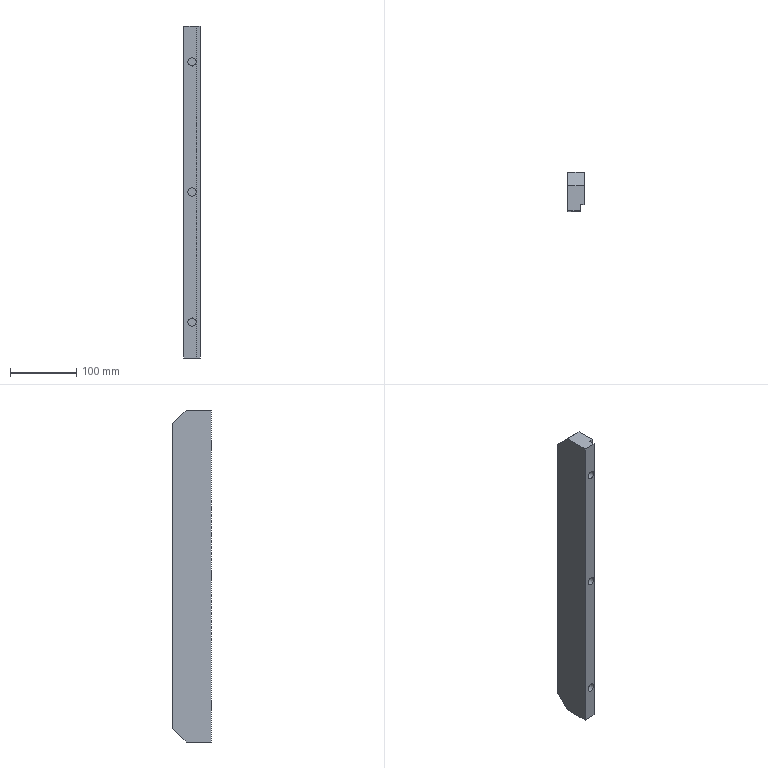Part | NX | 1 solid | 16 faces | box 25 x 58 x 500 mm | volume 672851 mm3 | plane 13 | cylinder 3 | commonest cylinder face diameters 12.5 x3
STEP:
#1=CARTESIAN_POINT('',(-12.5,29.,480.));
#2=VERTEX_POINT('',#1);
#3=CARTESIAN_POINT('',(-12.5,29.,20.));
#4=VERTEX_POINT('',#3);
#5=CARTESIAN_POINT('',(-12.5,29.,500.));
#6=DIRECTION('',(0.,0.,-1.));
#7=VECTOR('',#6,1000.);
#8=LINE('',#5,#7);
#9=EDGE_CURVE('',#2,#4,#8,.T.);
#10=ORIENTED_EDGE('',*,*,#9,.T.);
#11=CARTESIAN_POINT('',(-12.5,9.,0.));
#12=VERTEX_POINT('',#11);
#13=CARTESIAN_POINT('',(-12.5,29.,20.));
#14=DIRECTION('',(0.,0.7071,0.7071));
#15=VECTOR('',#14,1000.);
#16=LINE('',#13,#15);
#17=EDGE_CURVE('',#4,#12,#16,.F.);
#18=ORIENTED_EDGE('',*,*,#17,.T.);
#19=CARTESIAN_POINT('',(-12.5,-29.,0.));
#20=VERTEX_POINT('',#19);
#21=CARTESIAN_POINT('',(-12.5,29.,0.));
#22=DIRECTION('',(0.,-1.,0.));
#23=VECTOR('',#22,1000.);
#24=LINE('',#21,#23);
#25=EDGE_CURVE('',#12,#20,#24,.T.);
#26=ORIENTED_EDGE('',*,*,#25,.T.);
#27=CARTESIAN_POINT('',(-12.5,-29.,500.));
#28=VERTEX_POINT('',#27);
#29=CARTESIAN_POINT('',(-12.5,-29.,500.));
#30=DIRECTION('',(0.,0.,-1.));
#31=VECTOR('',#30,1000.);
#32=LINE('',#29,#31);
#33=EDGE_CURVE('',#28,#20,#32,.T.);
#34=ORIENTED_EDGE('',*,*,#33,.F.);
#35=CARTESIAN_POINT('',(-12.5,9.,500.));
#36=VERTEX_POINT('',#35);
#37=CARTESIAN_POINT('',(-12.5,29.,500.));
#38=DIRECTION('',(0.,-1.,0.));
#39=VECTOR('',#38,1000.);
#40=LINE('',#37,#39);
#41=EDGE_CURVE('',#36,#28,#40,.T.);
#42=ORIENTED_EDGE('',*,*,#41,.F.);
#43=CARTESIAN_POINT('',(-12.5,9.,500.));
#44=DIRECTION('',(0.,0.7071,-0.7071));
#45=VECTOR('',#44,1000.);
#46=LINE('',#43,#45);
#47=EDGE_CURVE('',#36,#2,#46,.T.);
#48=ORIENTED_EDGE('',*,*,#47,.T.);
#49=EDGE_LOOP('',(#10,#18,#26,#34,#42,#48));
#50=FACE_BOUND('',#49,.T.);
#51=CARTESIAN_POINT('',(-12.5,29.,500.));
#52=DIRECTION('',(1.,0.,0.));
#53=DIRECTION('',(0.,0.,-1.));
#54=AXIS2_PLACEMENT_3D('',#51,#52,#53);
#55=PLANE('',#54);
#56=ADVANCED_FACE('',(#50),#55,.F.);
#57=CARTESIAN_POINT('',(0.,-29.,452.25));
#58=VERTEX_POINT('',#57);
#59=CARTESIAN_POINT('',(0.,-29.,446.));
#60=DIRECTION('',(0.,-1.,0.));
#61=DIRECTION('',(0.,0.,1.));
#62=AXIS2_PLACEMENT_3D('',#59,#60,#61);
#63=CIRCLE('',#62,6.25);
#64=EDGE_CURVE('',#58,#58,#63,.T.);
#65=ORIENTED_EDGE('',*,*,#64,.F.);
#66=EDGE_LOOP('',(#65));
#67=FACE_BOUND('',#66,.T.);
#68=CARTESIAN_POINT('',(0.,-29.,60.25));
#69=VERTEX_POINT('',#68);
#70=CARTESIAN_POINT('',(0.,-29.,54.));
#71=DIRECTION('',(0.,-1.,0.));
#72=DIRECTION('',(0.,0.,1.));
#73=AXIS2_PLACEMENT_3D('',#70,#71,#72);
#74=CIRCLE('',#73,6.25);
#75=EDGE_CURVE('',#69,#69,#74,.T.);
#76=ORIENTED_EDGE('',*,*,#75,.F.);
#77=EDGE_LOOP('',(#76));
#78=FACE_BOUND('',#77,.T.);
#79=CARTESIAN_POINT('',(0.,-29.,256.25));
#80=VERTEX_POINT('',#79);
#81=CARTESIAN_POINT('',(0.,-29.,250.));
#82=DIRECTION('',(0.,-1.,0.));
#83=DIRECTION('',(0.,0.,1.));
#84=AXIS2_PLACEMENT_3D('',#81,#82,#83);
#85=CIRCLE('',#84,6.25);
#86=EDGE_CURVE('',#80,#80,#85,.T.);
#87=ORIENTED_EDGE('',*,*,#86,.F.);
#88=EDGE_LOOP('',(#87));
#89=FACE_BOUND('',#88,.T.);
#90=CARTESIAN_POINT('',(6.5,-29.,0.));
#91=VERTEX_POINT('',#90);
#92=CARTESIAN_POINT('',(-12.5,-29.,0.));
#93=DIRECTION('',(1.,0.,0.));
#94=VECTOR('',#93,1000.);
#95=LINE('',#92,#94);
#96=EDGE_CURVE('',#20,#91,#95,.T.);
#97=ORIENTED_EDGE('',*,*,#96,.T.);
#98=CARTESIAN_POINT('',(6.5,-29.,500.));
#99=VERTEX_POINT('',#98);
#100=CARTESIAN_POINT('',(6.5,-29.,500.));
#101=DIRECTION('',(0.,0.,-1.));
#102=VECTOR('',#101,1000.);
#103=LINE('',#100,#102);
#104=EDGE_CURVE('',#99,#91,#103,.T.);
#105=ORIENTED_EDGE('',*,*,#104,.F.);
#106=CARTESIAN_POINT('',(-12.5,-29.,500.));
#107=DIRECTION('',(1.,0.,0.));
#108=VECTOR('',#107,1000.);
#109=LINE('',#106,#108);
#110=EDGE_CURVE('',#28,#99,#109,.T.);
#111=ORIENTED_EDGE('',*,*,#110,.F.);
#112=ORIENTED_EDGE('',*,*,#33,.T.);
#113=EDGE_LOOP('',(#97,#105,#111,#112));
#114=FACE_BOUND('',#113,.T.);
#115=CARTESIAN_POINT('',(-12.5,-29.,500.));
#116=DIRECTION('',(0.,1.,0.));
#117=DIRECTION('',(0.,0.,1.));
#118=AXIS2_PLACEMENT_3D('',#115,#116,#117);
#119=PLANE('',#118);
#120=ADVANCED_FACE('',(#67,#78,#89,#114),#119,.F.);
#121=CARTESIAN_POINT('',(6.5,-19.,0.));
#122=VERTEX_POINT('',#121);
#123=CARTESIAN_POINT('',(6.5,-29.,0.));
#124=DIRECTION('',(0.,1.,0.));
#125=VECTOR('',#124,1000.);
#126=LINE('',#123,#125);
#127=EDGE_CURVE('',#91,#122,#126,.T.);
#128=ORIENTED_EDGE('',*,*,#127,.T.);
#129=CARTESIAN_POINT('',(6.5,-19.,500.));
#130=VERTEX_POINT('',#129);
#131=CARTESIAN_POINT('',(6.5,-19.,500.));
#132=DIRECTION('',(0.,0.,-1.));
#133=VECTOR('',#132,1000.);
#134=LINE('',#131,#133);
#135=EDGE_CURVE('',#130,#122,#134,.T.);
#136=ORIENTED_EDGE('',*,*,#135,.F.);
#137=CARTESIAN_POINT('',(6.5,-29.,500.));
#138=DIRECTION('',(0.,1.,0.));
#139=VECTOR('',#138,1000.);
#140=LINE('',#137,#139);
#141=EDGE_CURVE('',#99,#130,#140,.T.);
#142=ORIENTED_EDGE('',*,*,#141,.F.);
#143=ORIENTED_EDGE('',*,*,#104,.T.);
#144=EDGE_LOOP('',(#128,#136,#142,#143));
#145=FACE_BOUND('',#144,.T.);
#146=CARTESIAN_POINT('',(6.5,-29.,500.));
#147=DIRECTION('',(-1.,0.,0.));
#148=DIRECTION('',(0.,-1.,0.));
#149=AXIS2_PLACEMENT_3D('',#146,#147,#148);
#150=PLANE('',#149);
#151=ADVANCED_FACE('',(#145),#150,.F.);
#152=CARTESIAN_POINT('',(12.5,-19.,0.));
#153=VERTEX_POINT('',#152);
#154=CARTESIAN_POINT('',(6.5,-19.,0.));
#155=DIRECTION('',(1.,0.,0.));
#156=VECTOR('',#155,1000.);
#157=LINE('',#154,#156);
#158=EDGE_CURVE('',#122,#153,#157,.T.);
#159=ORIENTED_EDGE('',*,*,#158,.T.);
#160=CARTESIAN_POINT('',(12.5,-19.,500.));
#161=VERTEX_POINT('',#160);
#162=CARTESIAN_POINT('',(12.5,-19.,500.));
#163=DIRECTION('',(0.,0.,-1.));
#164=VECTOR('',#163,1000.);
#165=LINE('',#162,#164);
#166=EDGE_CURVE('',#161,#153,#165,.T.);
#167=ORIENTED_EDGE('',*,*,#166,.F.);
#168=CARTESIAN_POINT('',(6.5,-19.,500.));
#169=DIRECTION('',(1.,0.,0.));
#170=VECTOR('',#169,1000.);
#171=LINE('',#168,#170);
#172=EDGE_CURVE('',#130,#161,#171,.T.);
#173=ORIENTED_EDGE('',*,*,#172,.F.);
#174=ORIENTED_EDGE('',*,*,#135,.T.);
#175=EDGE_LOOP('',(#159,#167,#173,#174));
#176=FACE_BOUND('',#175,.T.);
#177=CARTESIAN_POINT('',(6.5,-19.,500.));
#178=DIRECTION('',(0.,1.,0.));
#179=DIRECTION('',(0.,0.,1.));
#180=AXIS2_PLACEMENT_3D('',#177,#178,#179);
#181=PLANE('',#180);
#182=ADVANCED_FACE('',(#176),#181,.F.);
#183=CARTESIAN_POINT('',(12.5,9.,0.));
#184=VERTEX_POINT('',#183);
#185=CARTESIAN_POINT('',(12.5,-19.,0.));
#186=DIRECTION('',(0.,1.,0.));
#187=VECTOR('',#186,1000.);
#188=LINE('',#185,#187);
#189=EDGE_CURVE('',#153,#184,#188,.T.);
#190=ORIENTED_EDGE('',*,*,#189,.T.);
#191=CARTESIAN_POINT('',(12.5,29.,20.));
#192=VERTEX_POINT('',#191);
#193=CARTESIAN_POINT('',(12.5,29.,20.));
#194=DIRECTION('',(0.,-0.7071,-0.7071));
#195=VECTOR('',#194,1000.);
#196=LINE('',#193,#195);
#197=EDGE_CURVE('',#184,#192,#196,.F.);
#198=ORIENTED_EDGE('',*,*,#197,.T.);
#199=CARTESIAN_POINT('',(12.5,29.,480.));
#200=VERTEX_POINT('',#199);
#201=CARTESIAN_POINT('',(12.5,29.,500.));
#202=DIRECTION('',(0.,0.,-1.));
#203=VECTOR('',#202,1000.);
#204=LINE('',#201,#203);
#205=EDGE_CURVE('',#200,#192,#204,.T.);
#206=ORIENTED_EDGE('',*,*,#205,.F.);
#207=CARTESIAN_POINT('',(12.5,9.,500.));
#208=VERTEX_POINT('',#207);
#209=CARTESIAN_POINT('',(12.5,9.,500.));
#210=DIRECTION('',(0.,-0.7071,0.7071));
#211=VECTOR('',#210,1000.);
#212=LINE('',#209,#211);
#213=EDGE_CURVE('',#200,#208,#212,.T.);
#214=ORIENTED_EDGE('',*,*,#213,.T.);
#215=CARTESIAN_POINT('',(12.5,-19.,500.));
#216=DIRECTION('',(0.,1.,0.));
#217=VECTOR('',#216,1000.);
#218=LINE('',#215,#217);
#219=EDGE_CURVE('',#161,#208,#218,.T.);
#220=ORIENTED_EDGE('',*,*,#219,.F.);
#221=ORIENTED_EDGE('',*,*,#166,.T.);
#222=EDGE_LOOP('',(#190,#198,#206,#214,#220,#221));
#223=FACE_BOUND('',#222,.T.);
#224=CARTESIAN_POINT('',(12.5,-19.,500.));
#225=DIRECTION('',(-1.,0.,0.));
#226=DIRECTION('',(0.,0.,1.));
#227=AXIS2_PLACEMENT_3D('',#224,#225,#226);
#228=PLANE('',#227);
#229=ADVANCED_FACE('',(#223),#228,.F.);
#230=ORIENTED_EDGE('',*,*,#205,.T.);
#231=CARTESIAN_POINT('',(12.5,29.,20.));
#232=DIRECTION('',(-1.,0.,0.));
#233=VECTOR('',#232,1000.);
#234=LINE('',#231,#233);
#235=EDGE_CURVE('',#192,#4,#234,.T.);
#236=ORIENTED_EDGE('',*,*,#235,.T.);
#237=ORIENTED_EDGE('',*,*,#9,.F.);
#238=CARTESIAN_POINT('',(12.5,29.,480.));
#239=DIRECTION('',(1.,0.,0.));
#240=VECTOR('',#239,1000.);
#241=LINE('',#238,#240);
#242=EDGE_CURVE('',#2,#200,#241,.T.);
#243=ORIENTED_EDGE('',*,*,#242,.T.);
#244=EDGE_LOOP('',(#230,#236,#237,#243));
#245=FACE_BOUND('',#244,.T.);
#246=CARTESIAN_POINT('',(12.5,29.,500.));
#247=DIRECTION('',(0.,-1.,0.));
#248=DIRECTION('',(0.,0.,-1.));
#249=AXIS2_PLACEMENT_3D('',#246,#247,#248);
#250=PLANE('',#249);
#251=ADVANCED_FACE('',(#245),#250,.F.);
#252=ORIENTED_EDGE('',*,*,#219,.T.);
#253=CARTESIAN_POINT('',(-12.5,9.,500.));
#254=DIRECTION('',(-1.,0.,0.));
#255=VECTOR('',#254,1000.);
#256=LINE('',#253,#255);
#257=EDGE_CURVE('',#208,#36,#256,.T.);
#258=ORIENTED_EDGE('',*,*,#257,.T.);
#259=ORIENTED_EDGE('',*,*,#41,.T.);
#260=ORIENTED_EDGE('',*,*,#110,.T.);
#261=ORIENTED_EDGE('',*,*,#141,.T.);
#262=ORIENTED_EDGE('',*,*,#172,.T.);
#263=EDGE_LOOP('',(#252,#258,#259,#260,#261,#262));
#264=FACE_BOUND('',#263,.T.);
#265=CARTESIAN_POINT('',(0.,0.,500.));
#266=DIRECTION('',(0.,0.,1.));
#267=DIRECTION('',(1.,0.,0.));
#268=AXIS2_PLACEMENT_3D('',#265,#266,#267);
#269=PLANE('',#268);
#270=ADVANCED_FACE('',(#264),#269,.T.);
#271=ORIENTED_EDGE('',*,*,#25,.F.);
#272=CARTESIAN_POINT('',(0.,9.,0.));
#273=DIRECTION('',(1.,0.,0.));
#274=VECTOR('',#273,1000.);
#275=LINE('',#272,#274);
#276=EDGE_CURVE('',#12,#184,#275,.T.);
#277=ORIENTED_EDGE('',*,*,#276,.T.);
#278=ORIENTED_EDGE('',*,*,#189,.F.);
#279=ORIENTED_EDGE('',*,*,#158,.F.);
#280=ORIENTED_EDGE('',*,*,#127,.F.);
#281=ORIENTED_EDGE('',*,*,#96,.F.);
#282=EDGE_LOOP('',(#271,#277,#278,#279,#280,#281));
#283=FACE_BOUND('',#282,.T.);
#284=CARTESIAN_POINT('',(0.,0.,0.));
#285=DIRECTION('',(0.,0.,1.));
#286=DIRECTION('',(1.,0.,0.));
#287=AXIS2_PLACEMENT_3D('',#284,#285,#286);
#288=PLANE('',#287);
#289=ADVANCED_FACE('',(#283),#288,.F.);
#290=ORIENTED_EDGE('',*,*,#197,.F.);
#291=ORIENTED_EDGE('',*,*,#276,.F.);
#292=ORIENTED_EDGE('',*,*,#17,.F.);
#293=ORIENTED_EDGE('',*,*,#235,.F.);
#294=EDGE_LOOP('',(#290,#291,#292,#293));
#295=FACE_BOUND('',#294,.T.);
#296=CARTESIAN_POINT('',(12.5,29.,20.));
#297=DIRECTION('',(0.,-0.7071,0.7071));
#298=DIRECTION('',(-1.,0.,0.));
#299=AXIS2_PLACEMENT_3D('',#296,#297,#298);
#300=PLANE('',#299);
#301=ADVANCED_FACE('',(#295),#300,.F.);
#302=ORIENTED_EDGE('',*,*,#213,.F.);
#303=ORIENTED_EDGE('',*,*,#242,.F.);
#304=ORIENTED_EDGE('',*,*,#47,.F.);
#305=ORIENTED_EDGE('',*,*,#257,.F.);
#306=EDGE_LOOP('',(#302,#303,#304,#305));
#307=FACE_BOUND('',#306,.T.);
#308=CARTESIAN_POINT('',(0.,9.,500.));
#309=DIRECTION('',(0.,0.7071,0.7071));
#310=DIRECTION('',(1.,0.,0.));
#311=AXIS2_PLACEMENT_3D('',#308,#309,#310);
#312=PLANE('',#311);
#313=ADVANCED_FACE('',(#307),#312,.T.);
#314=CARTESIAN_POINT('',(0.,4.,256.25));
#315=VERTEX_POINT('',#314);
#316=CARTESIAN_POINT('',(0.,4.,250.));
#317=DIRECTION('',(0.,-1.,0.));
#318=DIRECTION('',(0.,0.,1.));
#319=AXIS2_PLACEMENT_3D('',#316,#317,#318);
#320=CIRCLE('',#319,6.25);
#321=EDGE_CURVE('',#315,#315,#320,.F.);
#322=ORIENTED_EDGE('',*,*,#321,.T.);
#323=EDGE_LOOP('',(#322));
#324=FACE_BOUND('',#323,.T.);
#325=ORIENTED_EDGE('',*,*,#86,.T.);
#326=EDGE_LOOP('',(#325));
#327=FACE_BOUND('',#326,.T.);
#328=CARTESIAN_POINT('',(0.,4.,250.));
#329=DIRECTION('',(0.,-1.,0.));
#330=DIRECTION('',(0.,0.,-1.));
#331=AXIS2_PLACEMENT_3D('',#328,#329,#330);
#332=CYLINDRICAL_SURFACE('',#331,6.25);
#333=ADVANCED_FACE('',(#324,#327),#332,.F.);
#334=ORIENTED_EDGE('',*,*,#321,.F.);
#335=EDGE_LOOP('',(#334));
#336=FACE_BOUND('',#335,.T.);
#337=CARTESIAN_POINT('',(0.,4.,250.));
#338=DIRECTION('',(0.,-1.,0.));
#339=DIRECTION('',(0.,0.,-1.));
#340=AXIS2_PLACEMENT_3D('',#337,#338,#339);
#341=PLANE('',#340);
#342=ADVANCED_FACE('',(#336),#341,.T.);
#343=CARTESIAN_POINT('',(0.,4.,60.25));
#344=VERTEX_POINT('',#343);
#345=CARTESIAN_POINT('',(0.,4.,54.));
#346=DIRECTION('',(0.,-1.,0.));
#347=DIRECTION('',(0.,0.,1.));
#348=AXIS2_PLACEMENT_3D('',#345,#346,#347);
#349=CIRCLE('',#348,6.25);
#350=EDGE_CURVE('',#344,#344,#349,.F.);
#351=ORIENTED_EDGE('',*,*,#350,.T.);
#352=EDGE_LOOP('',(#351));
#353=FACE_BOUND('',#352,.T.);
#354=ORIENTED_EDGE('',*,*,#75,.T.);
#355=EDGE_LOOP('',(#354));
#356=FACE_BOUND('',#355,.T.);
#357=CARTESIAN_POINT('',(0.,4.,54.));
#358=DIRECTION('',(0.,-1.,0.));
#359=DIRECTION('',(0.,0.,-1.));
#360=AXIS2_PLACEMENT_3D('',#357,#358,#359);
#361=CYLINDRICAL_SURFACE('',#360,6.25);
#362=ADVANCED_FACE('',(#353,#356),#361,.F.);
#363=ORIENTED_EDGE('',*,*,#350,.F.);
#364=EDGE_LOOP('',(#363));
#365=FACE_BOUND('',#364,.T.);
#366=CARTESIAN_POINT('',(0.,4.,54.));
#367=DIRECTION('',(0.,-1.,0.));
#368=DIRECTION('',(0.,0.,-1.));
#369=AXIS2_PLACEMENT_3D('',#366,#367,#368);
#370=PLANE('',#369);
#371=ADVANCED_FACE('',(#365),#370,.T.);
#372=CARTESIAN_POINT('',(0.,4.,452.25));
#373=VERTEX_POINT('',#372);
#374=CARTESIAN_POINT('',(0.,4.,446.));
#375=DIRECTION('',(0.,-1.,0.));
#376=DIRECTION('',(0.,0.,1.));
#377=AXIS2_PLACEMENT_3D('',#374,#375,#376);
#378=CIRCLE('',#377,6.25);
#379=EDGE_CURVE('',#373,#373,#378,.F.);
#380=ORIENTED_EDGE('',*,*,#379,.T.);
#381=EDGE_LOOP('',(#380));
#382=FACE_BOUND('',#381,.T.);
#383=ORIENTED_EDGE('',*,*,#64,.T.);
#384=EDGE_LOOP('',(#383));
#385=FACE_BOUND('',#384,.T.);
#386=CARTESIAN_POINT('',(0.,4.,446.));
#387=DIRECTION('',(0.,-1.,0.));
#388=DIRECTION('',(0.,0.,-1.));
#389=AXIS2_PLACEMENT_3D('',#386,#387,#388);
#390=CYLINDRICAL_SURFACE('',#389,6.25);
#391=ADVANCED_FACE('',(#382,#385),#390,.F.);
#392=ORIENTED_EDGE('',*,*,#379,.F.);
#393=EDGE_LOOP('',(#392));
#394=FACE_BOUND('',#393,.T.);
#395=CARTESIAN_POINT('',(0.,4.,446.));
#396=DIRECTION('',(0.,-1.,0.));
#397=DIRECTION('',(0.,0.,-1.));
#398=AXIS2_PLACEMENT_3D('',#395,#396,#397);
#399=PLANE('',#398);
#400=ADVANCED_FACE('',(#394),#399,.T.);
#401=CLOSED_SHELL('',(#56,#120,#151,#182,#229,#251,#270,#289,#301,#313,#333,#342,#362,#371,#391,#400));
#402=MANIFOLD_SOLID_BREP('',#401);
#403=(LENGTH_UNIT()NAMED_UNIT(*)SI_UNIT(.MILLI.,.METRE.));
#404=UNCERTAINTY_MEASURE_WITH_UNIT(LENGTH_MEASURE(0.00001),#403,'','');
#405=(NAMED_UNIT(*)PLANE_ANGLE_UNIT()SI_UNIT($,.RADIAN.));
#406=(NAMED_UNIT(*)SI_UNIT($,.STERADIAN.)SOLID_ANGLE_UNIT());
#407=(GEOMETRIC_REPRESENTATION_CONTEXT(3)GLOBAL_UNCERTAINTY_ASSIGNED_CONTEXT((#404))GLOBAL_UNIT_ASSIGNED_CONTEXT((#403,#405,#406))REPRESENTATION_CONTEXT('',''));
#408=ADVANCED_BREP_SHAPE_REPRESENTATION('',(#402),#407);